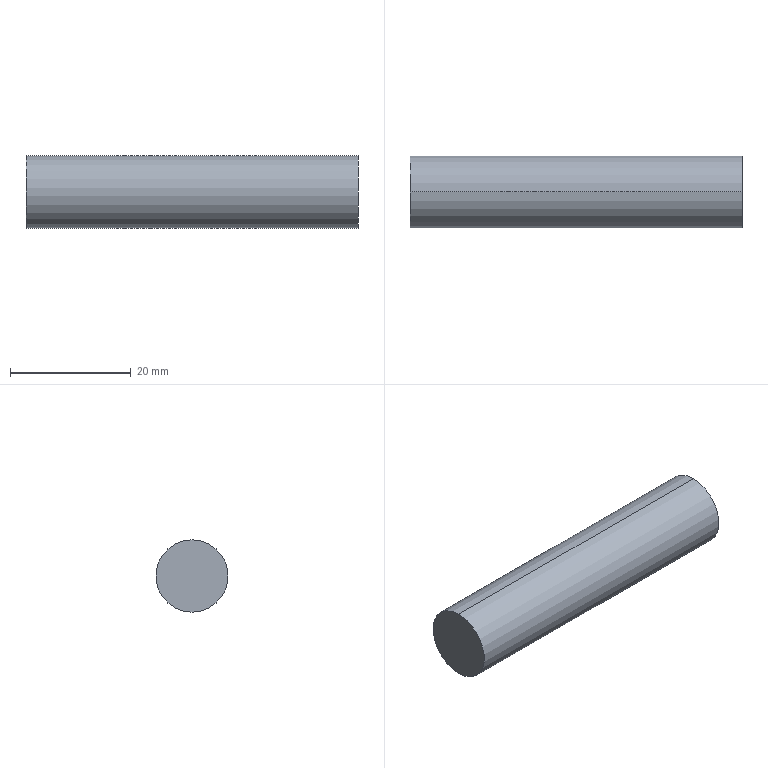Part | NX | features BREP 1 | 1 solid | 4 faces | box 55 x 12 x 12 mm | volume 6220 mm3 | cylinder 2 | plane 2 | commonest cylinder face diameters 12 x2
STEP:
#1=CARTESIAN_POINT('',(27.5,-3.,6.));
#2=VERTEX_POINT('',#1);
#3=CARTESIAN_POINT('',(27.5,-3.,-6.));
#4=VERTEX_POINT('',#3);
#5=CARTESIAN_POINT('',(27.5,-3.,0.));
#6=DIRECTION('',(-1.,0.,0.));
#7=DIRECTION('',(0.,0.,1.));
#8=AXIS2_PLACEMENT_3D('',#5,#6,#7);
#9=CIRCLE('',#8,6.);
#10=EDGE_CURVE('',#2,#4,#9,.T.);
#11=ORIENTED_EDGE('',*,*,#10,.T.);
#12=CARTESIAN_POINT('',(-27.5,-3.,-6.));
#13=VERTEX_POINT('',#12);
#14=CARTESIAN_POINT('',(-27.5,-3.,-6.));
#15=DIRECTION('',(-1.,0.,0.));
#16=VECTOR('',#15,1000.);
#17=LINE('',#14,#16);
#18=EDGE_CURVE('',#4,#13,#17,.T.);
#19=ORIENTED_EDGE('',*,*,#18,.T.);
#20=CARTESIAN_POINT('',(-27.5,-3.,6.));
#21=VERTEX_POINT('',#20);
#22=CARTESIAN_POINT('',(-27.5,-3.,0.));
#23=DIRECTION('',(-1.,0.,0.));
#24=DIRECTION('',(0.,0.,1.));
#25=AXIS2_PLACEMENT_3D('',#22,#23,#24);
#26=CIRCLE('',#25,6.);
#27=EDGE_CURVE('',#21,#13,#26,.T.);
#28=ORIENTED_EDGE('',*,*,#27,.F.);
#29=CARTESIAN_POINT('',(-27.5,-3.,6.));
#30=DIRECTION('',(-1.,0.,0.));
#31=VECTOR('',#30,1000.);
#32=LINE('',#29,#31);
#33=EDGE_CURVE('',#2,#21,#32,.T.);
#34=ORIENTED_EDGE('',*,*,#33,.F.);
#35=EDGE_LOOP('',(#11,#19,#28,#34));
#36=FACE_BOUND('',#35,.T.);
#37=CARTESIAN_POINT('',(-27.5,-3.,0.));
#38=DIRECTION('',(-1.,0.,0.));
#39=DIRECTION('',(0.,0.,-1.));
#40=AXIS2_PLACEMENT_3D('',#37,#38,#39);
#41=CYLINDRICAL_SURFACE('',#40,6.);
#42=ADVANCED_FACE('',(#36),#41,.T.);
#43=ORIENTED_EDGE('',*,*,#10,.F.);
#44=CARTESIAN_POINT('',(27.5,-3.,0.));
#45=DIRECTION('',(-1.,0.,0.));
#46=DIRECTION('',(0.,0.,1.));
#47=AXIS2_PLACEMENT_3D('',#44,#45,#46);
#48=CIRCLE('',#47,6.);
#49=EDGE_CURVE('',#4,#2,#48,.T.);
#50=ORIENTED_EDGE('',*,*,#49,.F.);
#51=EDGE_LOOP('',(#43,#50));
#52=FACE_BOUND('',#51,.T.);
#53=CARTESIAN_POINT('',(27.5,-3.,0.));
#54=DIRECTION('',(-1.,0.,0.));
#55=DIRECTION('',(0.,0.,-1.));
#56=AXIS2_PLACEMENT_3D('',#53,#54,#55);
#57=PLANE('',#56);
#58=ADVANCED_FACE('',(#52),#57,.F.);
#59=ORIENTED_EDGE('',*,*,#27,.T.);
#60=CARTESIAN_POINT('',(-27.5,-3.,0.));
#61=DIRECTION('',(-1.,0.,0.));
#62=DIRECTION('',(0.,0.,1.));
#63=AXIS2_PLACEMENT_3D('',#60,#61,#62);
#64=CIRCLE('',#63,6.);
#65=EDGE_CURVE('',#13,#21,#64,.T.);
#66=ORIENTED_EDGE('',*,*,#65,.T.);
#67=EDGE_LOOP('',(#59,#66));
#68=FACE_BOUND('',#67,.T.);
#69=CARTESIAN_POINT('',(-27.5,-3.,0.));
#70=DIRECTION('',(1.,0.,0.));
#71=DIRECTION('',(0.,-1.,0.));
#72=AXIS2_PLACEMENT_3D('',#69,#70,#71);
#73=PLANE('',#72);
#74=ADVANCED_FACE('',(#68),#73,.F.);
#75=ORIENTED_EDGE('',*,*,#18,.F.);
#76=ORIENTED_EDGE('',*,*,#49,.T.);
#77=ORIENTED_EDGE('',*,*,#33,.T.);
#78=ORIENTED_EDGE('',*,*,#65,.F.);
#79=EDGE_LOOP('',(#75,#76,#77,#78));
#80=FACE_BOUND('',#79,.T.);
#81=CARTESIAN_POINT('',(-27.5,-3.,0.));
#82=DIRECTION('',(-1.,0.,0.));
#83=DIRECTION('',(0.,0.,-1.));
#84=AXIS2_PLACEMENT_3D('',#81,#82,#83);
#85=CYLINDRICAL_SURFACE('',#84,6.);
#86=ADVANCED_FACE('',(#80),#85,.T.);
#87=CLOSED_SHELL('',(#42,#58,#74,#86));
#88=MANIFOLD_SOLID_BREP('',#87);
#89=(LENGTH_UNIT()NAMED_UNIT(*)SI_UNIT(.MILLI.,.METRE.));
#90=UNCERTAINTY_MEASURE_WITH_UNIT(LENGTH_MEASURE(0.00001),#89,'','');
#91=(NAMED_UNIT(*)PLANE_ANGLE_UNIT()SI_UNIT($,.RADIAN.));
#92=(NAMED_UNIT(*)SI_UNIT($,.STERADIAN.)SOLID_ANGLE_UNIT());
#93=(GEOMETRIC_REPRESENTATION_CONTEXT(3)GLOBAL_UNCERTAINTY_ASSIGNED_CONTEXT((#90))GLOBAL_UNIT_ASSIGNED_CONTEXT((#89,#91,#92))REPRESENTATION_CONTEXT('',''));
#94=ADVANCED_BREP_SHAPE_REPRESENTATION('',(#88),#93);